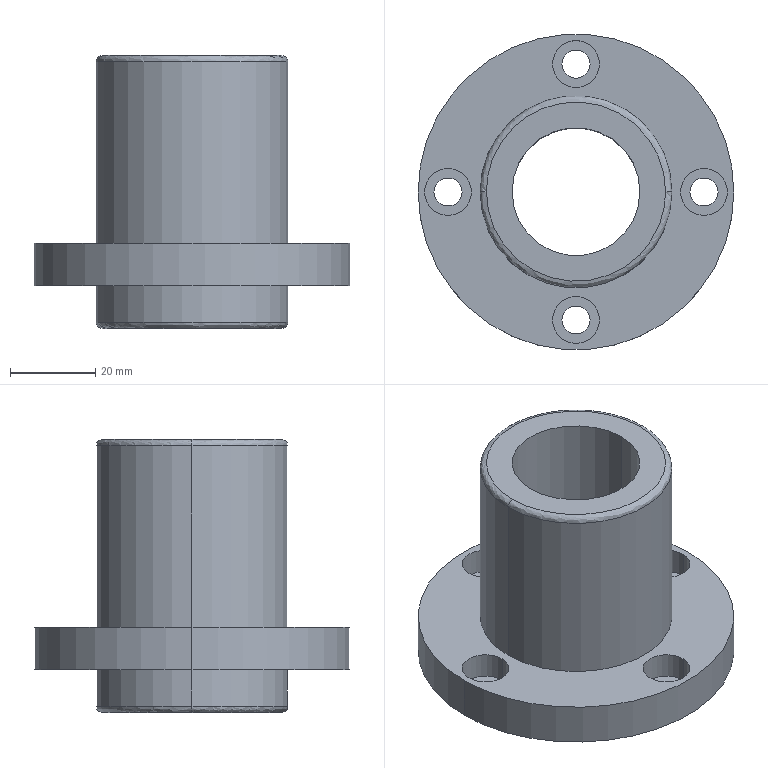Part | SolidWorks | features BaseBody 1 | 1 solid | 36 faces | box 74 x 74 x 64 mm | volume 80650 mm3 | cylinder 24 | plane 8 | spline 4 | commonest cylinder face diameters 6.6 x8 11 x8 45 x4 30 x2 74 x2